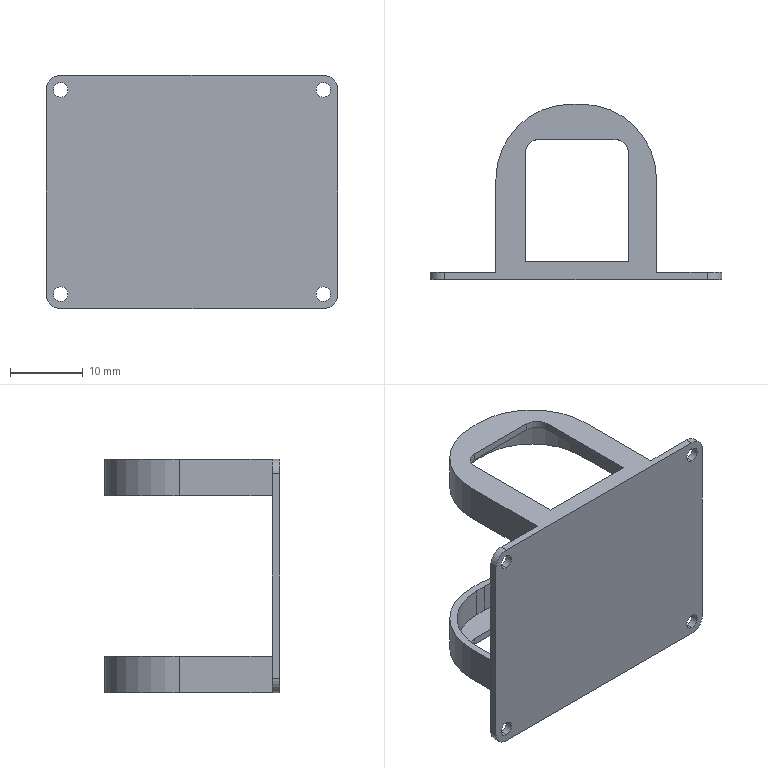Part | SolidWorks | features BaseBody 1 | 1 solid | 56 faces | box 40 x 24 x 32 mm | volume 2333 mm3 | plane 32 | cylinder 24 | commonest cylinder face diameters 2 x8 4 x8 18.5 x4 20.5 x4